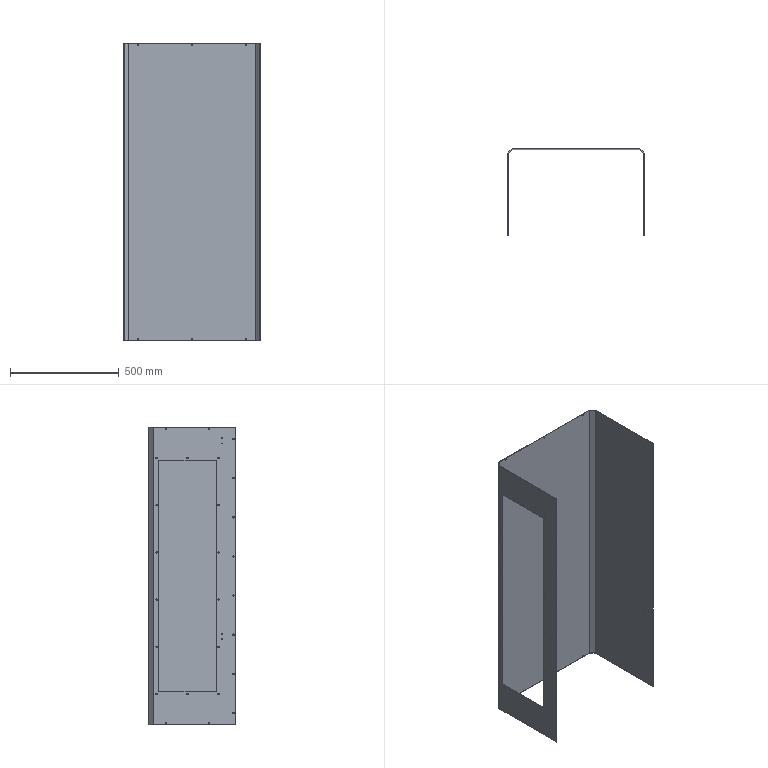Part | STEP file | 1 solid | 122 faces | box 628 x 396 x 1370 mm | volume 1949197 mm3 | cylinder 104 | plane 18 | commonest cylinder face diameters 6 x88 4.2 x16